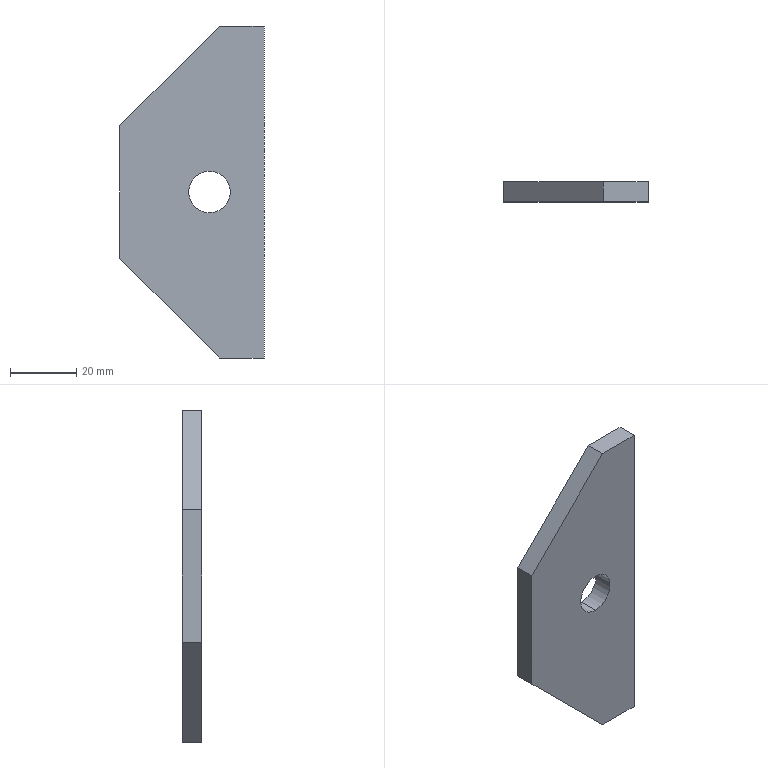Part | SolidWorks | features FlatPattern 1, SMBaseFlange 1, SheetMetal 1 | 1 solid | 10 faces | box 43.5 x 6 x 100 mm | volume 19964 mm3 | plane 8 | cylinder 2 | commonest cylinder face diameters 12.5 x2
STEP:
#1=CARTESIAN_POINT('',(-16.5,6.,-56.25));
#2=VERTEX_POINT('',#1);
#3=CARTESIAN_POINT('',(-16.5,6.,-43.75));
#4=VERTEX_POINT('',#3);
#5=CARTESIAN_POINT('',(-16.5,6.,-50.));
#6=DIRECTION('',(0.,1.,0.));
#7=DIRECTION('',(0.,0.,1.));
#8=AXIS2_PLACEMENT_3D('',#5,#6,#7);
#9=CIRCLE('',#8,6.25);
#10=EDGE_CURVE('',#2,#4,#9,.T.);
#11=ORIENTED_EDGE('',*,*,#10,.T.);
#12=CARTESIAN_POINT('',(-16.5,0.,-43.75));
#13=VERTEX_POINT('',#12);
#14=CARTESIAN_POINT('',(-16.5,6.,-43.75));
#15=DIRECTION('',(0.,-1.,0.));
#16=VECTOR('',#15,1000.);
#17=LINE('',#14,#16);
#18=EDGE_CURVE('',#4,#13,#17,.T.);
#19=ORIENTED_EDGE('',*,*,#18,.T.);
#20=CARTESIAN_POINT('',(-16.5,0.,-56.25));
#21=VERTEX_POINT('',#20);
#22=CARTESIAN_POINT('',(-16.5,0.,-50.));
#23=DIRECTION('',(0.,1.,0.));
#24=DIRECTION('',(0.,0.,1.));
#25=AXIS2_PLACEMENT_3D('',#22,#23,#24);
#26=CIRCLE('',#25,6.25);
#27=EDGE_CURVE('',#21,#13,#26,.T.);
#28=ORIENTED_EDGE('',*,*,#27,.F.);
#29=CARTESIAN_POINT('',(-16.5,6.,-56.25));
#30=DIRECTION('',(0.,-1.,0.));
#31=VECTOR('',#30,1000.);
#32=LINE('',#29,#31);
#33=EDGE_CURVE('',#2,#21,#32,.T.);
#34=ORIENTED_EDGE('',*,*,#33,.F.);
#35=EDGE_LOOP('',(#11,#19,#28,#34));
#36=FACE_OUTER_BOUND('',#35,.T.);
#37=CARTESIAN_POINT('',(-16.5,6.,-50.));
#38=DIRECTION('',(0.,-1.,0.));
#39=DIRECTION('',(0.,0.,-1.));
#40=AXIS2_PLACEMENT_3D('',#37,#38,#39);
#41=CYLINDRICAL_SURFACE('',#40,6.25);
#42=ADVANCED_FACE('',(#36),#41,.F.);
#43=CARTESIAN_POINT('',(0.,6.,0.));
#44=VERTEX_POINT('',#43);
#45=CARTESIAN_POINT('',(0.,6.,-100.));
#46=VERTEX_POINT('',#45);
#47=CARTESIAN_POINT('',(0.,6.,0.));
#48=DIRECTION('',(0.,0.,-1.));
#49=VECTOR('',#48,1000.);
#50=LINE('',#47,#49);
#51=EDGE_CURVE('',#44,#46,#50,.T.);
#52=ORIENTED_EDGE('',*,*,#51,.T.);
#53=CARTESIAN_POINT('',(-13.5,6.,-100.));
#54=VERTEX_POINT('',#53);
#55=CARTESIAN_POINT('',(0.,6.,-100.));
#56=DIRECTION('',(-1.,0.,0.));
#57=VECTOR('',#56,1000.);
#58=LINE('',#55,#57);
#59=EDGE_CURVE('',#46,#54,#58,.T.);
#60=ORIENTED_EDGE('',*,*,#59,.T.);
#61=CARTESIAN_POINT('',(-43.5,6.,-70.));
#62=VERTEX_POINT('',#61);
#63=CARTESIAN_POINT('',(-13.5,6.,-100.));
#64=DIRECTION('',(-0.7071,0.,0.7071));
#65=VECTOR('',#64,1000.);
#66=LINE('',#63,#65);
#67=EDGE_CURVE('',#54,#62,#66,.T.);
#68=ORIENTED_EDGE('',*,*,#67,.T.);
#69=CARTESIAN_POINT('',(-43.5,6.,-30.));
#70=VERTEX_POINT('',#69);
#71=CARTESIAN_POINT('',(-43.5,6.,-30.));
#72=DIRECTION('',(0.,0.,1.));
#73=VECTOR('',#72,1000.);
#74=LINE('',#71,#73);
#75=EDGE_CURVE('',#62,#70,#74,.T.);
#76=ORIENTED_EDGE('',*,*,#75,.T.);
#77=CARTESIAN_POINT('',(-13.5,6.,0.));
#78=VERTEX_POINT('',#77);
#79=CARTESIAN_POINT('',(-13.5,6.,0.));
#80=DIRECTION('',(0.7071,0.,0.7071));
#81=VECTOR('',#80,1000.);
#82=LINE('',#79,#81);
#83=EDGE_CURVE('',#70,#78,#82,.T.);
#84=ORIENTED_EDGE('',*,*,#83,.T.);
#85=CARTESIAN_POINT('',(0.,6.,0.));
#86=DIRECTION('',(1.,0.,0.));
#87=VECTOR('',#86,1000.);
#88=LINE('',#85,#87);
#89=EDGE_CURVE('',#78,#44,#88,.T.);
#90=ORIENTED_EDGE('',*,*,#89,.T.);
#91=EDGE_LOOP('',(#52,#60,#68,#76,#84,#90));
#92=FACE_OUTER_BOUND('',#91,.T.);
#93=ORIENTED_EDGE('',*,*,#10,.F.);
#94=CARTESIAN_POINT('',(-16.5,6.,-50.));
#95=DIRECTION('',(0.,1.,0.));
#96=DIRECTION('',(0.,0.,1.));
#97=AXIS2_PLACEMENT_3D('',#94,#95,#96);
#98=CIRCLE('',#97,6.25);
#99=EDGE_CURVE('',#4,#2,#98,.T.);
#100=ORIENTED_EDGE('',*,*,#99,.F.);
#101=EDGE_LOOP('',(#93,#100));
#102=FACE_BOUND('',#101,.T.);
#103=CARTESIAN_POINT('',(0.,6.,0.));
#104=DIRECTION('',(0.,1.,0.));
#105=DIRECTION('',(0.,0.,1.));
#106=AXIS2_PLACEMENT_3D('',#103,#104,#105);
#107=PLANE('',#106);
#108=ADVANCED_FACE('',(#92,#102),#107,.T.);
#109=CARTESIAN_POINT('',(0.,0.,0.));
#110=VERTEX_POINT('',#109);
#111=CARTESIAN_POINT('',(0.,0.,-100.));
#112=VERTEX_POINT('',#111);
#113=CARTESIAN_POINT('',(0.,0.,0.));
#114=DIRECTION('',(0.,0.,-1.));
#115=VECTOR('',#114,1000.);
#116=LINE('',#113,#115);
#117=EDGE_CURVE('',#110,#112,#116,.T.);
#118=ORIENTED_EDGE('',*,*,#117,.F.);
#119=CARTESIAN_POINT('',(-13.5,0.,0.));
#120=VERTEX_POINT('',#119);
#121=CARTESIAN_POINT('',(0.,0.,0.));
#122=DIRECTION('',(1.,0.,0.));
#123=VECTOR('',#122,1000.);
#124=LINE('',#121,#123);
#125=EDGE_CURVE('',#120,#110,#124,.T.);
#126=ORIENTED_EDGE('',*,*,#125,.F.);
#127=CARTESIAN_POINT('',(-43.5,0.,-30.));
#128=VERTEX_POINT('',#127);
#129=CARTESIAN_POINT('',(-13.5,0.,0.));
#130=DIRECTION('',(0.7071,0.,0.7071));
#131=VECTOR('',#130,1000.);
#132=LINE('',#129,#131);
#133=EDGE_CURVE('',#128,#120,#132,.T.);
#134=ORIENTED_EDGE('',*,*,#133,.F.);
#135=CARTESIAN_POINT('',(-43.5,0.,-70.));
#136=VERTEX_POINT('',#135);
#137=CARTESIAN_POINT('',(-43.5,0.,-30.));
#138=DIRECTION('',(0.,0.,1.));
#139=VECTOR('',#138,1000.);
#140=LINE('',#137,#139);
#141=EDGE_CURVE('',#136,#128,#140,.T.);
#142=ORIENTED_EDGE('',*,*,#141,.F.);
#143=CARTESIAN_POINT('',(-13.5,0.,-100.));
#144=VERTEX_POINT('',#143);
#145=CARTESIAN_POINT('',(-13.5,0.,-100.));
#146=DIRECTION('',(-0.7071,0.,0.7071));
#147=VECTOR('',#146,1000.);
#148=LINE('',#145,#147);
#149=EDGE_CURVE('',#144,#136,#148,.T.);
#150=ORIENTED_EDGE('',*,*,#149,.F.);
#151=CARTESIAN_POINT('',(0.,0.,-100.));
#152=DIRECTION('',(-1.,0.,0.));
#153=VECTOR('',#152,1000.);
#154=LINE('',#151,#153);
#155=EDGE_CURVE('',#112,#144,#154,.T.);
#156=ORIENTED_EDGE('',*,*,#155,.F.);
#157=EDGE_LOOP('',(#118,#126,#134,#142,#150,#156));
#158=FACE_OUTER_BOUND('',#157,.T.);
#159=ORIENTED_EDGE('',*,*,#27,.T.);
#160=CARTESIAN_POINT('',(-16.5,0.,-50.));
#161=DIRECTION('',(0.,1.,0.));
#162=DIRECTION('',(0.,0.,1.));
#163=AXIS2_PLACEMENT_3D('',#160,#161,#162);
#164=CIRCLE('',#163,6.25);
#165=EDGE_CURVE('',#13,#21,#164,.T.);
#166=ORIENTED_EDGE('',*,*,#165,.T.);
#167=EDGE_LOOP('',(#159,#166));
#168=FACE_BOUND('',#167,.T.);
#169=CARTESIAN_POINT('',(0.,0.,0.));
#170=DIRECTION('',(0.,1.,0.));
#171=DIRECTION('',(0.,0.,1.));
#172=AXIS2_PLACEMENT_3D('',#169,#170,#171);
#173=PLANE('',#172);
#174=ADVANCED_FACE('',(#158,#168),#173,.F.);
#175=ORIENTED_EDGE('',*,*,#117,.T.);
#176=CARTESIAN_POINT('',(0.,6.,-100.));
#177=DIRECTION('',(0.,-1.,0.));
#178=VECTOR('',#177,1000.);
#179=LINE('',#176,#178);
#180=EDGE_CURVE('',#46,#112,#179,.T.);
#181=ORIENTED_EDGE('',*,*,#180,.F.);
#182=ORIENTED_EDGE('',*,*,#51,.F.);
#183=CARTESIAN_POINT('',(0.,6.,0.));
#184=DIRECTION('',(0.,-1.,0.));
#185=VECTOR('',#184,1000.);
#186=LINE('',#183,#185);
#187=EDGE_CURVE('',#44,#110,#186,.T.);
#188=ORIENTED_EDGE('',*,*,#187,.T.);
#189=EDGE_LOOP('',(#175,#181,#182,#188));
#190=FACE_OUTER_BOUND('',#189,.T.);
#191=CARTESIAN_POINT('',(0.,6.,0.));
#192=DIRECTION('',(-1.,0.,0.));
#193=DIRECTION('',(0.,0.,1.));
#194=AXIS2_PLACEMENT_3D('',#191,#192,#193);
#195=PLANE('',#194);
#196=ADVANCED_FACE('',(#190),#195,.F.);
#197=ORIENTED_EDGE('',*,*,#155,.T.);
#198=CARTESIAN_POINT('',(-13.5,6.,-100.));
#199=DIRECTION('',(0.,-1.,0.));
#200=VECTOR('',#199,1000.);
#201=LINE('',#198,#200);
#202=EDGE_CURVE('',#54,#144,#201,.T.);
#203=ORIENTED_EDGE('',*,*,#202,.F.);
#204=ORIENTED_EDGE('',*,*,#59,.F.);
#205=ORIENTED_EDGE('',*,*,#180,.T.);
#206=EDGE_LOOP('',(#197,#203,#204,#205));
#207=FACE_OUTER_BOUND('',#206,.T.);
#208=CARTESIAN_POINT('',(0.,6.,-100.));
#209=DIRECTION('',(0.,0.,1.));
#210=DIRECTION('',(1.,0.,0.));
#211=AXIS2_PLACEMENT_3D('',#208,#209,#210);
#212=PLANE('',#211);
#213=ADVANCED_FACE('',(#207),#212,.F.);
#214=ORIENTED_EDGE('',*,*,#149,.T.);
#215=CARTESIAN_POINT('',(-43.5,6.,-70.));
#216=DIRECTION('',(0.,-1.,0.));
#217=VECTOR('',#216,1000.);
#218=LINE('',#215,#217);
#219=EDGE_CURVE('',#62,#136,#218,.T.);
#220=ORIENTED_EDGE('',*,*,#219,.F.);
#221=ORIENTED_EDGE('',*,*,#67,.F.);
#222=ORIENTED_EDGE('',*,*,#202,.T.);
#223=EDGE_LOOP('',(#214,#220,#221,#222));
#224=FACE_OUTER_BOUND('',#223,.T.);
#225=CARTESIAN_POINT('',(-13.5,6.,-100.));
#226=DIRECTION('',(0.7071,0.,0.7071));
#227=DIRECTION('',(0.7071,0.,-0.7071));
#228=AXIS2_PLACEMENT_3D('',#225,#226,#227);
#229=PLANE('',#228);
#230=ADVANCED_FACE('',(#224),#229,.F.);
#231=ORIENTED_EDGE('',*,*,#141,.T.);
#232=CARTESIAN_POINT('',(-43.5,6.,-30.));
#233=DIRECTION('',(0.,-1.,0.));
#234=VECTOR('',#233,1000.);
#235=LINE('',#232,#234);
#236=EDGE_CURVE('',#70,#128,#235,.T.);
#237=ORIENTED_EDGE('',*,*,#236,.F.);
#238=ORIENTED_EDGE('',*,*,#75,.F.);
#239=ORIENTED_EDGE('',*,*,#219,.T.);
#240=EDGE_LOOP('',(#231,#237,#238,#239));
#241=FACE_OUTER_BOUND('',#240,.T.);
#242=CARTESIAN_POINT('',(-43.5,6.,-30.));
#243=DIRECTION('',(1.,0.,0.));
#244=DIRECTION('',(0.,0.,-1.));
#245=AXIS2_PLACEMENT_3D('',#242,#243,#244);
#246=PLANE('',#245);
#247=ADVANCED_FACE('',(#241),#246,.F.);
#248=ORIENTED_EDGE('',*,*,#133,.T.);
#249=CARTESIAN_POINT('',(-13.5,6.,0.));
#250=DIRECTION('',(0.,-1.,0.));
#251=VECTOR('',#250,1000.);
#252=LINE('',#249,#251);
#253=EDGE_CURVE('',#78,#120,#252,.T.);
#254=ORIENTED_EDGE('',*,*,#253,.F.);
#255=ORIENTED_EDGE('',*,*,#83,.F.);
#256=ORIENTED_EDGE('',*,*,#236,.T.);
#257=EDGE_LOOP('',(#248,#254,#255,#256));
#258=FACE_OUTER_BOUND('',#257,.T.);
#259=CARTESIAN_POINT('',(-13.5,6.,0.));
#260=DIRECTION('',(0.7071,0.,-0.7071));
#261=DIRECTION('',(-0.7071,0.,-0.7071));
#262=AXIS2_PLACEMENT_3D('',#259,#260,#261);
#263=PLANE('',#262);
#264=ADVANCED_FACE('',(#258),#263,.F.);
#265=ORIENTED_EDGE('',*,*,#125,.T.);
#266=ORIENTED_EDGE('',*,*,#187,.F.);
#267=ORIENTED_EDGE('',*,*,#89,.F.);
#268=ORIENTED_EDGE('',*,*,#253,.T.);
#269=EDGE_LOOP('',(#265,#266,#267,#268));
#270=FACE_OUTER_BOUND('',#269,.T.);
#271=CARTESIAN_POINT('',(0.,6.,0.));
#272=DIRECTION('',(0.,0.,-1.));
#273=DIRECTION('',(-1.,0.,0.));
#274=AXIS2_PLACEMENT_3D('',#271,#272,#273);
#275=PLANE('',#274);
#276=ADVANCED_FACE('',(#270),#275,.F.);
#277=ORIENTED_EDGE('',*,*,#18,.F.);
#278=ORIENTED_EDGE('',*,*,#99,.T.);
#279=ORIENTED_EDGE('',*,*,#33,.T.);
#280=ORIENTED_EDGE('',*,*,#165,.F.);
#281=EDGE_LOOP('',(#277,#278,#279,#280));
#282=FACE_OUTER_BOUND('',#281,.T.);
#283=CARTESIAN_POINT('',(-16.5,6.,-50.));
#284=DIRECTION('',(0.,-1.,0.));
#285=DIRECTION('',(0.,0.,-1.));
#286=AXIS2_PLACEMENT_3D('',#283,#284,#285);
#287=CYLINDRICAL_SURFACE('',#286,6.25);
#288=ADVANCED_FACE('',(#282),#287,.F.);
#289=CLOSED_SHELL('',(#42,#108,#174,#196,#213,#230,#247,#264,#276,#288));
#290=MANIFOLD_SOLID_BREP('',#289);
#291=CARTESIAN_POINT('',(0.,0.,0.));
#292=DIRECTION('',(0.,0.,1.));
#293=DIRECTION('',(1.,0.,0.));
#294=AXIS2_PLACEMENT_3D('',#291,#292,#293);
#295=(LENGTH_UNIT()NAMED_UNIT(*)SI_UNIT(.MILLI.,.METRE.));
#296=UNCERTAINTY_MEASURE_WITH_UNIT(LENGTH_MEASURE(0.00001),#295,'','');
#297=(NAMED_UNIT(*)PLANE_ANGLE_UNIT()SI_UNIT($,.RADIAN.));
#298=(NAMED_UNIT(*)SI_UNIT($,.STERADIAN.)SOLID_ANGLE_UNIT());
#299=(GEOMETRIC_REPRESENTATION_CONTEXT(3)GLOBAL_UNCERTAINTY_ASSIGNED_CONTEXT((#296))GLOBAL_UNIT_ASSIGNED_CONTEXT((#295,#297,#298))REPRESENTATION_CONTEXT('',''));
#300=ADVANCED_BREP_SHAPE_REPRESENTATION('',(#290,#294),#299);